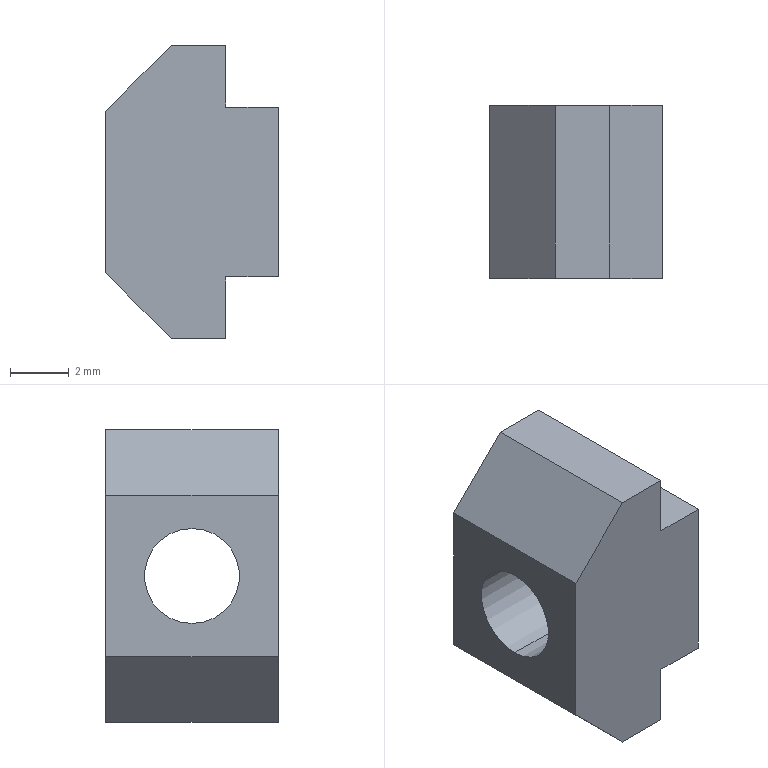Part | STEP file | PN_0018_T-slot nut M4 | 1 solid | 16 faces | box 5.9 x 5.9 x 10 mm | volume 224.64 mm3 | plane 12 | cylinder 2 | cone 2 | commonest cylinder face diameters 3.242 x2
STEP:
#1=CARTESIAN_POINT('',(0.,0.,0.));
#2=DIRECTION('',(0.,0.,1.));
#3=DIRECTION('',(1.,0.,0.));
#4=AXIS2_PLACEMENT_3D('',#1,#2,#3);
#5=CARTESIAN_POINT('',(-3770.9,379.188,502.528));
#6=VERTEX_POINT('',#5);
#7=CARTESIAN_POINT('',(-3765.219,379.188,502.528));
#8=VERTEX_POINT('',#7);
#9=CARTESIAN_POINT('',(-3765.,379.188,502.528));
#10=DIRECTION('',(1.,0.,0.));
#11=VECTOR('',#10,1.);
#12=LINE('',#9,#11);
#13=CARTESIAN_POINT('',(-3765.,379.188,504.149));
#14=DIRECTION('',(1.,0.,0.));
#15=DIRECTION('',(0.,0.,-1.));
#16=AXIS2_PLACEMENT_3D('',#13,#14,#15);
#17=CYLINDRICAL_SURFACE('',#16,1.621);
#18=CARTESIAN_POINT('',(6.283,0.));
#19=DIRECTION('',(0.,1.));
#20=VECTOR('',#19,1.);
#21=LINE('',#18,#20);
#22=(GEOMETRIC_REPRESENTATION_CONTEXT(2)PARAMETRIC_REPRESENTATION_CONTEXT()REPRESENTATION_CONTEXT('',''));
#23=DEFINITIONAL_REPRESENTATION('',(#21),#22);
#24=PCURVE('',#17,#23);
#25=CARTESIAN_POINT('',(-3765.,379.188,504.149));
#26=DIRECTION('',(1.,0.,0.));
#27=DIRECTION('',(0.,0.,-1.));
#28=AXIS2_PLACEMENT_3D('',#25,#26,#27);
#29=CYLINDRICAL_SURFACE('',#28,1.621);
#30=CARTESIAN_POINT('',(0.,0.));
#31=DIRECTION('',(0.,1.));
#32=VECTOR('',#31,1.);
#33=LINE('',#30,#32);
#34=(GEOMETRIC_REPRESENTATION_CONTEXT(2)PARAMETRIC_REPRESENTATION_CONTEXT()REPRESENTATION_CONTEXT('',''));
#35=DEFINITIONAL_REPRESENTATION('',(#33),#34);
#36=PCURVE('',#29,#35);
#37=SURFACE_CURVE('',#12,(#24,#36),.PCURVE_S1.);
#38=EDGE_CURVE('',#6,#8,#37,.T.);
#39=ORIENTED_EDGE('',*,*,#38,.T.);
#40=CARTESIAN_POINT('',(-3765.219,379.188,505.77));
#41=VERTEX_POINT('',#40);
#42=CARTESIAN_POINT('',(-3765.219,379.188,504.149));
#43=DIRECTION('',(-1.,0.,0.));
#44=DIRECTION('',(0.,0.,-1.));
#45=AXIS2_PLACEMENT_3D('',#42,#43,#44);
#46=CIRCLE('',#45,1.621);
#47=CARTESIAN_POINT('',(6.283,-0.2188));
#48=DIRECTION('',(-1.,0.));
#49=VECTOR('',#48,1.);
#50=LINE('',#47,#49);
#51=(GEOMETRIC_REPRESENTATION_CONTEXT(2)PARAMETRIC_REPRESENTATION_CONTEXT()REPRESENTATION_CONTEXT('',''));
#52=DEFINITIONAL_REPRESENTATION('',(#50),#51);
#53=PCURVE('',#17,#52);
#54=CARTESIAN_POINT('',(-3765.,379.188,504.149));
#55=DIRECTION('',(1.,0.,0.));
#56=DIRECTION('',(0.,0.,-1.));
#57=AXIS2_PLACEMENT_3D('',#54,#55,#56);
#58=CONICAL_SURFACE('',#57,2.,1.047);
#59=CARTESIAN_POINT('',(6.283,-0.2188));
#60=DIRECTION('',(-1.,0.));
#61=VECTOR('',#60,1.);
#62=LINE('',#59,#61);
#63=(GEOMETRIC_REPRESENTATION_CONTEXT(2)PARAMETRIC_REPRESENTATION_CONTEXT()REPRESENTATION_CONTEXT('',''));
#64=DEFINITIONAL_REPRESENTATION('',(#62),#63);
#65=PCURVE('',#58,#64);
#66=SURFACE_CURVE('',#46,(#53,#65),.PCURVE_S1.);
#67=EDGE_CURVE('',#8,#41,#66,.T.);
#68=ORIENTED_EDGE('',*,*,#67,.T.);
#69=CARTESIAN_POINT('',(-3770.9,379.188,505.77));
#70=VERTEX_POINT('',#69);
#71=CARTESIAN_POINT('',(-3765.,379.188,505.77));
#72=DIRECTION('',(1.,0.,0.));
#73=VECTOR('',#72,1.);
#74=LINE('',#71,#73);
#75=CARTESIAN_POINT('',(3.142,0.));
#76=DIRECTION('',(0.,1.));
#77=VECTOR('',#76,1.);
#78=LINE('',#75,#77);
#79=(GEOMETRIC_REPRESENTATION_CONTEXT(2)PARAMETRIC_REPRESENTATION_CONTEXT()REPRESENTATION_CONTEXT('',''));
#80=DEFINITIONAL_REPRESENTATION('',(#78),#79);
#81=PCURVE('',#17,#80);
#82=CARTESIAN_POINT('',(3.142,0.));
#83=DIRECTION('',(0.,1.));
#84=VECTOR('',#83,1.);
#85=LINE('',#82,#84);
#86=(GEOMETRIC_REPRESENTATION_CONTEXT(2)PARAMETRIC_REPRESENTATION_CONTEXT()REPRESENTATION_CONTEXT('',''));
#87=DEFINITIONAL_REPRESENTATION('',(#85),#86);
#88=PCURVE('',#29,#87);
#89=SURFACE_CURVE('',#74,(#81,#88),.PCURVE_S1.);
#90=EDGE_CURVE('',#70,#41,#89,.T.);
#91=ORIENTED_EDGE('',*,*,#90,.F.);
#92=CARTESIAN_POINT('',(-3770.9,379.188,504.149));
#93=DIRECTION('',(1.,0.,0.));
#94=DIRECTION('',(0.,0.,-1.));
#95=AXIS2_PLACEMENT_3D('',#92,#93,#94);
#96=CIRCLE('',#95,1.621);
#97=CARTESIAN_POINT('',(0.,-5.9));
#98=DIRECTION('',(1.,0.));
#99=VECTOR('',#98,1.);
#100=LINE('',#97,#99);
#101=(GEOMETRIC_REPRESENTATION_CONTEXT(2)PARAMETRIC_REPRESENTATION_CONTEXT()REPRESENTATION_CONTEXT('',''));
#102=DEFINITIONAL_REPRESENTATION('',(#100),#101);
#103=PCURVE('',#17,#102);
#104=CARTESIAN_POINT('',(-3770.9,376.238,501.392));
#105=DIRECTION('',(-1.,0.,0.));
#106=DIRECTION('',(0.,0.,1.));
#107=AXIS2_PLACEMENT_3D('',#104,#105,#106);
#108=PLANE('',#107);
#109=CARTESIAN_POINT('',(1.135,2.95));
#110=CARTESIAN_POINT('',(1.135,5.758));
#111=CARTESIAN_POINT('',(3.567,4.354));
#112=CARTESIAN_POINT('',(5.998,2.95));
#113=CARTESIAN_POINT('',(3.567,1.546));
#114=CARTESIAN_POINT('',(1.135,0.1423));
#115=CARTESIAN_POINT('',(1.135,2.95));
#116=(BOUNDED_CURVE()B_SPLINE_CURVE(2,(#109,#110,#111,#112,#113,#114,#115),.UNSPECIFIED.,.T.,.F.)B_SPLINE_CURVE_WITH_KNOTS((1,2,2,2,2,1),(-2.094,0.,2.094,4.189,6.283,8.378),.UNSPECIFIED.)CURVE()GEOMETRIC_REPRESENTATION_ITEM()RATIONAL_B_SPLINE_CURVE((1.,0.5,1.,0.5,1.,0.5,1.))REPRESENTATION_ITEM(''));
#117=(GEOMETRIC_REPRESENTATION_CONTEXT(2)PARAMETRIC_REPRESENTATION_CONTEXT()REPRESENTATION_CONTEXT('',''));
#118=DEFINITIONAL_REPRESENTATION('',(#116),#117);
#119=PCURVE('',#108,#118);
#120=SURFACE_CURVE('',#96,(#103,#119),.PCURVE_S1.);
#121=EDGE_CURVE('',#70,#6,#120,.T.);
#122=ORIENTED_EDGE('',*,*,#121,.T.);
#123=EDGE_LOOP('',(#39,#68,#91,#122));
#124=FACE_BOUND('',#123,.F.);
#125=ADVANCED_FACE('',(#124),#17,.F.);
#126=CARTESIAN_POINT('',(-3765.,379.188,502.149));
#127=VERTEX_POINT('',#126);
#128=CARTESIAN_POINT('',(-3765.,379.188,502.149));
#129=DIRECTION('',(0.5,0.,-0.866));
#130=VECTOR('',#129,1.);
#131=LINE('',#128,#130);
#132=CARTESIAN_POINT('',(6.283,0.));
#133=DIRECTION('',(0.,1.));
#134=VECTOR('',#133,1.);
#135=LINE('',#132,#134);
#136=(GEOMETRIC_REPRESENTATION_CONTEXT(2)PARAMETRIC_REPRESENTATION_CONTEXT()REPRESENTATION_CONTEXT('',''));
#137=DEFINITIONAL_REPRESENTATION('',(#135),#136);
#138=PCURVE('',#58,#137);
#139=CARTESIAN_POINT('',(-3765.,379.188,504.149));
#140=DIRECTION('',(1.,0.,0.));
#141=DIRECTION('',(0.,0.,-1.));
#142=AXIS2_PLACEMENT_3D('',#139,#140,#141);
#143=CONICAL_SURFACE('',#142,2.,1.047);
#144=CARTESIAN_POINT('',(0.,0.));
#145=DIRECTION('',(0.,1.));
#146=VECTOR('',#145,1.);
#147=LINE('',#144,#146);
#148=(GEOMETRIC_REPRESENTATION_CONTEXT(2)PARAMETRIC_REPRESENTATION_CONTEXT()REPRESENTATION_CONTEXT('',''));
#149=DEFINITIONAL_REPRESENTATION('',(#147),#148);
#150=PCURVE('',#143,#149);
#151=SURFACE_CURVE('',#131,(#138,#150),.PCURVE_S1.);
#152=EDGE_CURVE('',#8,#127,#151,.T.);
#153=ORIENTED_EDGE('',*,*,#152,.T.);
#154=CARTESIAN_POINT('',(-3765.,379.188,506.149));
#155=VERTEX_POINT('',#154);
#156=CARTESIAN_POINT('',(-3765.,379.188,504.149));
#157=DIRECTION('',(-1.,0.,0.));
#158=DIRECTION('',(0.,0.,-1.));
#159=AXIS2_PLACEMENT_3D('',#156,#157,#158);
#160=CIRCLE('',#159,2.);
#161=CARTESIAN_POINT('',(6.283,0.));
#162=DIRECTION('',(-1.,0.));
#163=VECTOR('',#162,1.);
#164=LINE('',#161,#163);
#165=(GEOMETRIC_REPRESENTATION_CONTEXT(2)PARAMETRIC_REPRESENTATION_CONTEXT()REPRESENTATION_CONTEXT('',''));
#166=DEFINITIONAL_REPRESENTATION('',(#164),#165);
#167=PCURVE('',#58,#166);
#168=CARTESIAN_POINT('',(-3765.,376.238,509.149));
#169=DIRECTION('',(1.,0.,0.));
#170=DIRECTION('',(0.,0.,-1.));
#171=AXIS2_PLACEMENT_3D('',#168,#169,#170);
#172=PLANE('',#171);
#173=CARTESIAN_POINT('',(7.,2.95));
#174=CARTESIAN_POINT('',(7.,-0.5141));
#175=CARTESIAN_POINT('',(4.,1.218));
#176=CARTESIAN_POINT('',(1.,2.95));
#177=CARTESIAN_POINT('',(4.,4.682));
#178=CARTESIAN_POINT('',(7.,6.414));
#179=CARTESIAN_POINT('',(7.,2.95));
#180=(BOUNDED_CURVE()B_SPLINE_CURVE(2,(#173,#174,#175,#176,#177,#178,#179),.UNSPECIFIED.,.T.,.F.)B_SPLINE_CURVE_WITH_KNOTS((1,2,2,2,2,1),(-2.094,0.,2.094,4.189,6.283,8.378),.UNSPECIFIED.)CURVE()GEOMETRIC_REPRESENTATION_ITEM()RATIONAL_B_SPLINE_CURVE((1.,0.5,1.,0.5,1.,0.5,1.))REPRESENTATION_ITEM(''));
#181=(GEOMETRIC_REPRESENTATION_CONTEXT(2)PARAMETRIC_REPRESENTATION_CONTEXT()REPRESENTATION_CONTEXT('',''));
#182=DEFINITIONAL_REPRESENTATION('',(#180),#181);
#183=PCURVE('',#172,#182);
#184=SURFACE_CURVE('',#160,(#167,#183),.PCURVE_S1.);
#185=EDGE_CURVE('',#127,#155,#184,.T.);
#186=ORIENTED_EDGE('',*,*,#185,.T.);
#187=CARTESIAN_POINT('',(-3765.,379.188,506.149));
#188=DIRECTION('',(0.5,0.,0.866));
#189=VECTOR('',#188,1.);
#190=LINE('',#187,#189);
#191=CARTESIAN_POINT('',(3.142,0.));
#192=DIRECTION('',(0.,1.));
#193=VECTOR('',#192,1.);
#194=LINE('',#191,#193);
#195=(GEOMETRIC_REPRESENTATION_CONTEXT(2)PARAMETRIC_REPRESENTATION_CONTEXT()REPRESENTATION_CONTEXT('',''));
#196=DEFINITIONAL_REPRESENTATION('',(#194),#195);
#197=PCURVE('',#58,#196);
#198=CARTESIAN_POINT('',(3.142,0.));
#199=DIRECTION('',(0.,1.));
#200=VECTOR('',#199,1.);
#201=LINE('',#198,#200);
#202=(GEOMETRIC_REPRESENTATION_CONTEXT(2)PARAMETRIC_REPRESENTATION_CONTEXT()REPRESENTATION_CONTEXT('',''));
#203=DEFINITIONAL_REPRESENTATION('',(#201),#202);
#204=PCURVE('',#143,#203);
#205=SURFACE_CURVE('',#190,(#197,#204),.PCURVE_S1.);
#206=EDGE_CURVE('',#41,#155,#205,.T.);
#207=ORIENTED_EDGE('',*,*,#206,.F.);
#208=ORIENTED_EDGE('',*,*,#67,.F.);
#209=EDGE_LOOP('',(#153,#186,#207,#208));
#210=FACE_BOUND('',#209,.F.);
#211=ADVANCED_FACE('',(#210),#58,.F.);
#212=CARTESIAN_POINT('',(-3768.656,376.238,499.149));
#213=VERTEX_POINT('',#212);
#214=CARTESIAN_POINT('',(-3766.8,376.238,499.149));
#215=VERTEX_POINT('',#214);
#216=CARTESIAN_POINT('',(0.,376.238,499.149));
#217=DIRECTION('',(1.,0.,0.));
#218=VECTOR('',#217,1.);
#219=LINE('',#216,#218);
#220=CARTESIAN_POINT('',(0.,376.238,0.));
#221=DIRECTION('',(0.,-1.,0.));
#222=DIRECTION('',(0.,0.,-1.));
#223=AXIS2_PLACEMENT_3D('',#220,#221,#222);
#224=PLANE('',#223);
#225=CARTESIAN_POINT('',(-499.149,0.));
#226=DIRECTION('',(0.,1.));
#227=VECTOR('',#226,1.);
#228=LINE('',#225,#227);
#229=(GEOMETRIC_REPRESENTATION_CONTEXT(2)PARAMETRIC_REPRESENTATION_CONTEXT()REPRESENTATION_CONTEXT('',''));
#230=DEFINITIONAL_REPRESENTATION('',(#228),#229);
#231=PCURVE('',#224,#230);
#232=CARTESIAN_POINT('',(-3765.,376.238,499.149));
#233=DIRECTION('',(0.,0.,-1.));
#234=DIRECTION('',(-1.,0.,0.));
#235=AXIS2_PLACEMENT_3D('',#232,#233,#234);
#236=PLANE('',#235);
#237=CARTESIAN_POINT('',(-3765.,0.));
#238=DIRECTION('',(-1.,0.));
#239=VECTOR('',#238,1.);
#240=LINE('',#237,#239);
#241=(GEOMETRIC_REPRESENTATION_CONTEXT(2)PARAMETRIC_REPRESENTATION_CONTEXT()REPRESENTATION_CONTEXT('',''));
#242=DEFINITIONAL_REPRESENTATION('',(#240),#241);
#243=PCURVE('',#236,#242);
#244=SURFACE_CURVE('',#219,(#231,#243),.PCURVE_S1.);
#245=EDGE_CURVE('',#213,#215,#244,.T.);
#246=ORIENTED_EDGE('',*,*,#245,.T.);
#247=CARTESIAN_POINT('',(-3766.8,376.238,501.249));
#248=VERTEX_POINT('',#247);
#249=CARTESIAN_POINT('',(-3766.8,376.238,0.));
#250=DIRECTION('',(0.,0.,1.));
#251=VECTOR('',#250,1.);
#252=LINE('',#249,#251);
#253=CARTESIAN_POINT('',(0.,-3766.8));
#254=DIRECTION('',(-1.,0.));
#255=VECTOR('',#254,1.);
#256=LINE('',#253,#255);
#257=(GEOMETRIC_REPRESENTATION_CONTEXT(2)PARAMETRIC_REPRESENTATION_CONTEXT()REPRESENTATION_CONTEXT('',''));
#258=DEFINITIONAL_REPRESENTATION('',(#256),#257);
#259=PCURVE('',#224,#258);
#260=CARTESIAN_POINT('',(-3766.8,382.138,501.249));
#261=DIRECTION('',(-1.,0.,0.));
#262=DIRECTION('',(0.,0.,1.));
#263=AXIS2_PLACEMENT_3D('',#260,#261,#262);
#264=PLANE('',#263);
#265=CARTESIAN_POINT('',(-501.249,-5.9));
#266=DIRECTION('',(1.,0.));
#267=VECTOR('',#266,1.);
#268=LINE('',#265,#267);
#269=(GEOMETRIC_REPRESENTATION_CONTEXT(2)PARAMETRIC_REPRESENTATION_CONTEXT()REPRESENTATION_CONTEXT('',''));
#270=DEFINITIONAL_REPRESENTATION('',(#268),#269);
#271=PCURVE('',#264,#270);
#272=SURFACE_CURVE('',#252,(#259,#271),.PCURVE_S1.);
#273=EDGE_CURVE('',#215,#248,#272,.T.);
#274=ORIENTED_EDGE('',*,*,#273,.T.);
#275=CARTESIAN_POINT('',(-3765.,376.238,501.249));
#276=VERTEX_POINT('',#275);
#277=CARTESIAN_POINT('',(0.,376.238,501.249));
#278=DIRECTION('',(1.,0.,0.));
#279=VECTOR('',#278,1.);
#280=LINE('',#277,#279);
#281=CARTESIAN_POINT('',(-501.249,0.));
#282=DIRECTION('',(0.,1.));
#283=VECTOR('',#282,1.);
#284=LINE('',#281,#283);
#285=(GEOMETRIC_REPRESENTATION_CONTEXT(2)PARAMETRIC_REPRESENTATION_CONTEXT()REPRESENTATION_CONTEXT('',''));
#286=DEFINITIONAL_REPRESENTATION('',(#284),#285);
#287=PCURVE('',#224,#286);
#288=CARTESIAN_POINT('',(-3765.,382.138,501.249));
#289=DIRECTION('',(0.,0.,1.));
#290=DIRECTION('',(1.,0.,0.));
#291=AXIS2_PLACEMENT_3D('',#288,#289,#290);
#292=PLANE('',#291);
#293=CARTESIAN_POINT('',(3765.,-5.9));
#294=DIRECTION('',(1.,0.));
#295=VECTOR('',#294,1.);
#296=LINE('',#293,#295);
#297=(GEOMETRIC_REPRESENTATION_CONTEXT(2)PARAMETRIC_REPRESENTATION_CONTEXT()REPRESENTATION_CONTEXT('',''));
#298=DEFINITIONAL_REPRESENTATION('',(#296),#297);
#299=PCURVE('',#292,#298);
#300=SURFACE_CURVE('',#280,(#287,#299),.PCURVE_S1.);
#301=EDGE_CURVE('',#248,#276,#300,.T.);
#302=ORIENTED_EDGE('',*,*,#301,.T.);
#303=CARTESIAN_POINT('',(-3765.,376.238,507.049));
#304=VERTEX_POINT('',#303);
#305=CARTESIAN_POINT('',(-3765.,376.238,0.));
#306=DIRECTION('',(0.,0.,1.));
#307=VECTOR('',#306,1.);
#308=LINE('',#305,#307);
#309=CARTESIAN_POINT('',(0.,-3765.));
#310=DIRECTION('',(-1.,0.));
#311=VECTOR('',#310,1.);
#312=LINE('',#309,#311);
#313=(GEOMETRIC_REPRESENTATION_CONTEXT(2)PARAMETRIC_REPRESENTATION_CONTEXT()REPRESENTATION_CONTEXT('',''));
#314=DEFINITIONAL_REPRESENTATION('',(#312),#313);
#315=PCURVE('',#224,#314);
#316=CARTESIAN_POINT('',(509.149,0.));
#317=DIRECTION('',(-1.,0.));
#318=VECTOR('',#317,1.);
#319=LINE('',#316,#318);
#320=(GEOMETRIC_REPRESENTATION_CONTEXT(2)PARAMETRIC_REPRESENTATION_CONTEXT()REPRESENTATION_CONTEXT('',''));
#321=DEFINITIONAL_REPRESENTATION('',(#319),#320);
#322=PCURVE('',#172,#321);
#323=SURFACE_CURVE('',#308,(#315,#322),.PCURVE_S1.);
#324=EDGE_CURVE('',#276,#304,#323,.T.);
#325=ORIENTED_EDGE('',*,*,#324,.T.);
#326=CARTESIAN_POINT('',(-3766.8,376.238,507.049));
#327=VERTEX_POINT('',#326);
#328=CARTESIAN_POINT('',(0.,376.238,507.049));
#329=DIRECTION('',(-1.,0.,0.));
#330=VECTOR('',#329,1.);
#331=LINE('',#328,#330);
#332=CARTESIAN_POINT('',(-507.049,0.));
#333=DIRECTION('',(0.,-1.));
#334=VECTOR('',#333,1.);
#335=LINE('',#332,#334);
#336=(GEOMETRIC_REPRESENTATION_CONTEXT(2)PARAMETRIC_REPRESENTATION_CONTEXT()REPRESENTATION_CONTEXT('',''));
#337=DEFINITIONAL_REPRESENTATION('',(#335),#336);
#338=PCURVE('',#224,#337);
#339=CARTESIAN_POINT('',(-3766.8,382.138,507.049));
#340=DIRECTION('',(0.,0.,-1.));
#341=DIRECTION('',(-1.,0.,0.));
#342=AXIS2_PLACEMENT_3D('',#339,#340,#341);
#343=PLANE('',#342);
#344=CARTESIAN_POINT('',(-3766.8,-5.9));
#345=DIRECTION('',(1.,0.));
#346=VECTOR('',#345,1.);
#347=LINE('',#344,#346);
#348=(GEOMETRIC_REPRESENTATION_CONTEXT(2)PARAMETRIC_REPRESENTATION_CONTEXT()REPRESENTATION_CONTEXT('',''));
#349=DEFINITIONAL_REPRESENTATION('',(#347),#348);
#350=PCURVE('',#343,#349);
#351=SURFACE_CURVE('',#331,(#338,#350),.PCURVE_S1.);
#352=EDGE_CURVE('',#304,#327,#351,.T.);
#353=ORIENTED_EDGE('',*,*,#352,.T.);
#354=CARTESIAN_POINT('',(-3766.8,376.238,509.149));
#355=VERTEX_POINT('',#354);
#356=CARTESIAN_POINT('',(-3766.8,376.238,0.));
#357=DIRECTION('',(0.,0.,1.));
#358=VECTOR('',#357,1.);
#359=LINE('',#356,#358);
#360=CARTESIAN_POINT('',(0.,-3766.8));
#361=DIRECTION('',(-1.,0.));
#362=VECTOR('',#361,1.);
#363=LINE('',#360,#362);
#364=(GEOMETRIC_REPRESENTATION_CONTEXT(2)PARAMETRIC_REPRESENTATION_CONTEXT()REPRESENTATION_CONTEXT('',''));
#365=DEFINITIONAL_REPRESENTATION('',(#363),#364);
#366=PCURVE('',#224,#365);
#367=CARTESIAN_POINT('',(-3766.8,382.138,509.149));
#368=DIRECTION('',(-1.,0.,0.));
#369=DIRECTION('',(0.,0.,1.));
#370=AXIS2_PLACEMENT_3D('',#367,#368,#369);
#371=PLANE('',#370);
#372=CARTESIAN_POINT('',(-509.149,-5.9));
#373=DIRECTION('',(1.,0.));
#374=VECTOR('',#373,1.);
#375=LINE('',#372,#374);
#376=(GEOMETRIC_REPRESENTATION_CONTEXT(2)PARAMETRIC_REPRESENTATION_CONTEXT()REPRESENTATION_CONTEXT('',''));
#377=DEFINITIONAL_REPRESENTATION('',(#375),#376);
#378=PCURVE('',#371,#377);
#379=SURFACE_CURVE('',#359,(#366,#378),.PCURVE_S1.);
#380=EDGE_CURVE('',#327,#355,#379,.T.);
#381=ORIENTED_EDGE('',*,*,#380,.T.);
#382=CARTESIAN_POINT('',(-3768.656,376.238,509.149));
#383=VERTEX_POINT('',#382);
#384=CARTESIAN_POINT('',(0.,376.238,509.149));
#385=DIRECTION('',(-1.,0.,0.));
#386=VECTOR('',#385,1.);
#387=LINE('',#384,#386);
#388=CARTESIAN_POINT('',(-509.149,0.));
#389=DIRECTION('',(0.,-1.));
#390=VECTOR('',#389,1.);
#391=LINE('',#388,#390);
#392=(GEOMETRIC_REPRESENTATION_CONTEXT(2)PARAMETRIC_REPRESENTATION_CONTEXT()REPRESENTATION_CONTEXT('',''));
#393=DEFINITIONAL_REPRESENTATION('',(#391),#392);
#394=PCURVE('',#224,#393);
#395=CARTESIAN_POINT('',(-3768.656,376.238,509.149));
#396=DIRECTION('',(0.,0.,1.));
#397=DIRECTION('',(1.,0.,0.));
#398=AXIS2_PLACEMENT_3D('',#395,#396,#397);
#399=PLANE('',#398);
#400=CARTESIAN_POINT('',(3768.656,0.));
#401=DIRECTION('',(-1.,0.));
#402=VECTOR('',#401,1.);
#403=LINE('',#400,#402);
#404=(GEOMETRIC_REPRESENTATION_CONTEXT(2)PARAMETRIC_REPRESENTATION_CONTEXT()REPRESENTATION_CONTEXT('',''));
#405=DEFINITIONAL_REPRESENTATION('',(#403),#404);
#406=PCURVE('',#399,#405);
#407=SURFACE_CURVE('',#387,(#394,#406),.PCURVE_S1.);
#408=EDGE_CURVE('',#355,#383,#407,.T.);
#409=ORIENTED_EDGE('',*,*,#408,.T.);
#410=CARTESIAN_POINT('',(-3770.9,376.238,506.905));
#411=VERTEX_POINT('',#410);
#412=CARTESIAN_POINT('',(-3768.656,376.238,509.149));
#413=DIRECTION('',(-0.7071,0.,-0.7071));
#414=VECTOR('',#413,1.);
#415=LINE('',#412,#414);
#416=CARTESIAN_POINT('',(-509.149,-3768.656));
#417=DIRECTION('',(0.7071,-0.7071));
#418=VECTOR('',#417,1.);
#419=LINE('',#416,#418);
#420=(GEOMETRIC_REPRESENTATION_CONTEXT(2)PARAMETRIC_REPRESENTATION_CONTEXT()REPRESENTATION_CONTEXT('',''));
#421=DEFINITIONAL_REPRESENTATION('',(#419),#420);
#422=PCURVE('',#224,#421);
#423=CARTESIAN_POINT('',(-3770.9,376.238,506.905));
#424=DIRECTION('',(-0.7071,0.,0.7071));
#425=DIRECTION('',(0.7071,0.,0.7071));
#426=AXIS2_PLACEMENT_3D('',#423,#424,#425);
#427=PLANE('',#426);
#428=CARTESIAN_POINT('',(3.173,0.));
#429=DIRECTION('',(-1.,0.));
#430=VECTOR('',#429,1.);
#431=LINE('',#428,#430);
#432=(GEOMETRIC_REPRESENTATION_CONTEXT(2)PARAMETRIC_REPRESENTATION_CONTEXT()REPRESENTATION_CONTEXT('',''));
#433=DEFINITIONAL_REPRESENTATION('',(#431),#432);
#434=PCURVE('',#427,#433);
#435=SURFACE_CURVE('',#415,(#422,#434),.PCURVE_S1.);
#436=EDGE_CURVE('',#383,#411,#435,.T.);
#437=ORIENTED_EDGE('',*,*,#436,.T.);
#438=CARTESIAN_POINT('',(-3770.9,376.238,501.392));
#439=VERTEX_POINT('',#438);
#440=CARTESIAN_POINT('',(-3770.9,376.238,0.));
#441=DIRECTION('',(0.,0.,-1.));
#442=VECTOR('',#441,1.);
#443=LINE('',#440,#442);
#444=CARTESIAN_POINT('',(0.,-3770.9));
#445=DIRECTION('',(1.,0.));
#446=VECTOR('',#445,1.);
#447=LINE('',#444,#446);
#448=(GEOMETRIC_REPRESENTATION_CONTEXT(2)PARAMETRIC_REPRESENTATION_CONTEXT()REPRESENTATION_CONTEXT('',''));
#449=DEFINITIONAL_REPRESENTATION('',(#447),#448);
#450=PCURVE('',#224,#449);
#451=CARTESIAN_POINT('',(-501.392,0.));
#452=DIRECTION('',(-1.,0.));
#453=VECTOR('',#452,1.);
#454=LINE('',#451,#453);
#455=(GEOMETRIC_REPRESENTATION_CONTEXT(2)PARAMETRIC_REPRESENTATION_CONTEXT()REPRESENTATION_CONTEXT('',''));
#456=DEFINITIONAL_REPRESENTATION('',(#454),#455);
#457=PCURVE('',#108,#456);
#458=SURFACE_CURVE('',#443,(#450,#457),.PCURVE_S1.);
#459=EDGE_CURVE('',#411,#439,#458,.T.);
#460=ORIENTED_EDGE('',*,*,#459,.T.);
#461=CARTESIAN_POINT('',(-3770.9,376.238,501.392));
#462=DIRECTION('',(0.7071,0.,-0.7071));
#463=VECTOR('',#462,1.);
#464=LINE('',#461,#463);
#465=CARTESIAN_POINT('',(-501.392,-3770.9));
#466=DIRECTION('',(0.7071,0.7071));
#467=VECTOR('',#466,1.);
#468=LINE('',#465,#467);
#469=(GEOMETRIC_REPRESENTATION_CONTEXT(2)PARAMETRIC_REPRESENTATION_CONTEXT()REPRESENTATION_CONTEXT('',''));
#470=DEFINITIONAL_REPRESENTATION('',(#468),#469);
#471=PCURVE('',#224,#470);
#472=CARTESIAN_POINT('',(-3768.656,376.238,499.149));
#473=DIRECTION('',(-0.7071,0.,-0.7071));
#474=DIRECTION('',(-0.7071,0.,0.7071));
#475=AXIS2_PLACEMENT_3D('',#472,#473,#474);
#476=PLANE('',#475);
#477=CARTESIAN_POINT('',(3.173,0.));
#478=DIRECTION('',(-1.,0.));
#479=VECTOR('',#478,1.);
#480=LINE('',#477,#479);
#481=(GEOMETRIC_REPRESENTATION_CONTEXT(2)PARAMETRIC_REPRESENTATION_CONTEXT()REPRESENTATION_CONTEXT('',''));
#482=DEFINITIONAL_REPRESENTATION('',(#480),#481);
#483=PCURVE('',#476,#482);
#484=SURFACE_CURVE('',#464,(#471,#483),.PCURVE_S1.);
#485=EDGE_CURVE('',#439,#213,#484,.T.);
#486=ORIENTED_EDGE('',*,*,#485,.T.);
#487=EDGE_LOOP('',(#246,#274,#302,#325,#353,#381,#409,#437,#460,#486));
#488=FACE_BOUND('',#487,.T.);
#489=ADVANCED_FACE('',(#488),#224,.T.);
#490=CARTESIAN_POINT('',(-3766.8,382.138,499.149));
#491=VERTEX_POINT('',#490);
#492=CARTESIAN_POINT('',(-3766.8,382.138,499.149));
#493=DIRECTION('',(0.,-1.,0.));
#494=VECTOR('',#493,1.);
#495=LINE('',#492,#494);
#496=CARTESIAN_POINT('',(-2.1,0.));
#497=DIRECTION('',(0.,-1.));
#498=VECTOR('',#497,1.);
#499=LINE('',#496,#498);
#500=(GEOMETRIC_REPRESENTATION_CONTEXT(2)PARAMETRIC_REPRESENTATION_CONTEXT()REPRESENTATION_CONTEXT('',''));
#501=DEFINITIONAL_REPRESENTATION('',(#499),#500);
#502=PCURVE('',#264,#501);
#503=CARTESIAN_POINT('',(1.8,5.9));
#504=DIRECTION('',(0.,-1.));
#505=VECTOR('',#504,1.);
#506=LINE('',#503,#505);
#507=(GEOMETRIC_REPRESENTATION_CONTEXT(2)PARAMETRIC_REPRESENTATION_CONTEXT()REPRESENTATION_CONTEXT('',''));
#508=DEFINITIONAL_REPRESENTATION('',(#506),#507);
#509=PCURVE('',#236,#508);
#510=SURFACE_CURVE('',#495,(#502,#509),.PCURVE_S1.);
#511=EDGE_CURVE('',#491,#215,#510,.T.);
#512=ORIENTED_EDGE('',*,*,#511,.F.);
#513=CARTESIAN_POINT('',(-3766.8,382.138,501.249));
#514=VERTEX_POINT('',#513);
#515=CARTESIAN_POINT('',(-3766.8,382.138,501.249));
#516=DIRECTION('',(0.,0.,-1.));
#517=VECTOR('',#516,1.);
#518=LINE('',#515,#517);
#519=CARTESIAN_POINT('',(0.,0.));
#520=DIRECTION('',(-1.,0.));
#521=VECTOR('',#520,1.);
#522=LINE('',#519,#521);
#523=(GEOMETRIC_REPRESENTATION_CONTEXT(2)PARAMETRIC_REPRESENTATION_CONTEXT()REPRESENTATION_CONTEXT('',''));
#524=DEFINITIONAL_REPRESENTATION('',(#522),#523);
#525=PCURVE('',#264,#524);
#526=CARTESIAN_POINT('',(0.,382.138,0.));
#527=DIRECTION('',(0.,-1.,0.));
#528=DIRECTION('',(0.,0.,-1.));
#529=AXIS2_PLACEMENT_3D('',#526,#527,#528);
#530=PLANE('',#529);
#531=CARTESIAN_POINT('',(-501.249,-3766.8));
#532=DIRECTION('',(1.,0.));
#533=VECTOR('',#532,1.);
#534=LINE('',#531,#533);
#535=(GEOMETRIC_REPRESENTATION_CONTEXT(2)PARAMETRIC_REPRESENTATION_CONTEXT()REPRESENTATION_CONTEXT('',''));
#536=DEFINITIONAL_REPRESENTATION('',(#534),#535);
#537=PCURVE('',#530,#536);
#538=SURFACE_CURVE('',#518,(#525,#537),.PCURVE_S1.);
#539=EDGE_CURVE('',#514,#491,#538,.T.);
#540=ORIENTED_EDGE('',*,*,#539,.F.);
#541=CARTESIAN_POINT('',(-3766.8,382.138,501.249));
#542=DIRECTION('',(0.,1.,0.));
#543=VECTOR('',#542,1.);
#544=LINE('',#541,#543);
#545=CARTESIAN_POINT('',(0.,0.));
#546=DIRECTION('',(0.,1.));
#547=VECTOR('',#546,1.);
#548=LINE('',#545,#547);
#549=(GEOMETRIC_REPRESENTATION_CONTEXT(2)PARAMETRIC_REPRESENTATION_CONTEXT()REPRESENTATION_CONTEXT('',''));
#550=DEFINITIONAL_REPRESENTATION('',(#548),#549);
#551=PCURVE('',#264,#550);
#552=CARTESIAN_POINT('',(-1.8,0.));
#553=DIRECTION('',(0.,1.));
#554=VECTOR('',#553,1.);
#555=LINE('',#552,#554);
#556=(GEOMETRIC_REPRESENTATION_CONTEXT(2)PARAMETRIC_REPRESENTATION_CONTEXT()REPRESENTATION_CONTEXT('',''));
#557=DEFINITIONAL_REPRESENTATION('',(#555),#556);
#558=PCURVE('',#292,#557);
#559=SURFACE_CURVE('',#544,(#551,#558),.PCURVE_S1.);
#560=EDGE_CURVE('',#248,#514,#559,.T.);
#561=ORIENTED_EDGE('',*,*,#560,.F.);
#562=ORIENTED_EDGE('',*,*,#273,.F.);
#563=EDGE_LOOP('',(#512,#540,#561,#562));
#564=FACE_BOUND('',#563,.T.);
#565=ADVANCED_FACE('',(#564),#264,.F.);
#566=CARTESIAN_POINT('',(-3768.656,382.138,499.149));
#567=VERTEX_POINT('',#566);
#568=CARTESIAN_POINT('',(-3768.656,376.238,499.149));
#569=DIRECTION('',(0.,1.,0.));
#570=VECTOR('',#569,1.);
#571=LINE('',#568,#570);
#572=CARTESIAN_POINT('',(3.656,0.));
#573=DIRECTION('',(0.,1.));
#574=VECTOR('',#573,1.);
#575=LINE('',#572,#574);
#576=(GEOMETRIC_REPRESENTATION_CONTEXT(2)PARAMETRIC_REPRESENTATION_CONTEXT()REPRESENTATION_CONTEXT('',''));
#577=DEFINITIONAL_REPRESENTATION('',(#575),#576);
#578=PCURVE('',#236,#577);
#579=CARTESIAN_POINT('',(0.,0.));
#580=DIRECTION('',(0.,1.));
#581=VECTOR('',#580,1.);
#582=LINE('',#579,#581);
#583=(GEOMETRIC_REPRESENTATION_CONTEXT(2)PARAMETRIC_REPRESENTATION_CONTEXT()REPRESENTATION_CONTEXT('',''));
#584=DEFINITIONAL_REPRESENTATION('',(#582),#583);
#585=PCURVE('',#476,#584);
#586=SURFACE_CURVE('',#571,(#578,#585),.PCURVE_S1.);
#587=EDGE_CURVE('',#213,#567,#586,.T.);
#588=ORIENTED_EDGE('',*,*,#587,.T.);
#589=CARTESIAN_POINT('',(-3765.,382.138,499.149));
#590=DIRECTION('',(1.,0.,0.));
#591=VECTOR('',#590,1.);
#592=LINE('',#589,#591);
#593=CARTESIAN_POINT('',(0.,5.9));
#594=DIRECTION('',(-1.,0.));
#595=VECTOR('',#594,1.);
#596=LINE('',#593,#595);
#597=(GEOMETRIC_REPRESENTATION_CONTEXT(2)PARAMETRIC_REPRESENTATION_CONTEXT()REPRESENTATION_CONTEXT('',''));
#598=DEFINITIONAL_REPRESENTATION('',(#596),#597);
#599=PCURVE('',#236,#598);
#600=CARTESIAN_POINT('',(-499.149,-3765.));
#601=DIRECTION('',(0.,1.));
#602=VECTOR('',#601,1.);
#603=LINE('',#600,#602);
#604=(GEOMETRIC_REPRESENTATION_CONTEXT(2)PARAMETRIC_REPRESENTATION_CONTEXT()REPRESENTATION_CONTEXT('',''));
#605=DEFINITIONAL_REPRESENTATION('',(#603),#604);
#606=PCURVE('',#530,#605);
#607=SURFACE_CURVE('',#592,(#599,#606),.PCURVE_S1.);
#608=EDGE_CURVE('',#567,#491,#607,.T.);
#609=ORIENTED_EDGE('',*,*,#608,.T.);
#610=ORIENTED_EDGE('',*,*,#511,.T.);
#611=ORIENTED_EDGE('',*,*,#245,.F.);
#612=EDGE_LOOP('',(#588,#609,#610,#611));
#613=FACE_BOUND('',#612,.T.);
#614=ADVANCED_FACE('',(#613),#236,.T.);
#615=ORIENTED_EDGE('',*,*,#485,.F.);
#616=CARTESIAN_POINT('',(-3770.9,382.138,501.392));
#617=VERTEX_POINT('',#616);
#618=CARTESIAN_POINT('',(-3770.9,376.238,501.392));
#619=DIRECTION('',(0.,1.,0.));
#620=VECTOR('',#619,1.);
#621=LINE('',#618,#620);
#622=CARTESIAN_POINT('',(3.173,0.));
#623=DIRECTION('',(0.,1.));
#624=VECTOR('',#623,1.);
#625=LINE('',#622,#624);
#626=(GEOMETRIC_REPRESENTATION_CONTEXT(2)PARAMETRIC_REPRESENTATION_CONTEXT()REPRESENTATION_CONTEXT('',''));
#627=DEFINITIONAL_REPRESENTATION('',(#625),#626);
#628=PCURVE('',#476,#627);
#629=CARTESIAN_POINT('',(0.,0.));
#630=DIRECTION('',(0.,1.));
#631=VECTOR('',#630,1.);
#632=LINE('',#629,#631);
#633=(GEOMETRIC_REPRESENTATION_CONTEXT(2)PARAMETRIC_REPRESENTATION_CONTEXT()REPRESENTATION_CONTEXT('',''));
#634=DEFINITIONAL_REPRESENTATION('',(#632),#633);
#635=PCURVE('',#108,#634);
#636=SURFACE_CURVE('',#621,(#628,#635),.PCURVE_S1.);
#637=EDGE_CURVE('',#439,#617,#636,.T.);
#638=ORIENTED_EDGE('',*,*,#637,.T.);
#639=CARTESIAN_POINT('',(-3768.656,382.138,499.149));
#640=DIRECTION('',(0.7071,0.,-0.7071));
#641=VECTOR('',#640,1.);
#642=LINE('',#639,#641);
#643=CARTESIAN_POINT('',(0.,5.9));
#644=DIRECTION('',(-1.,0.));
#645=VECTOR('',#644,1.);
#646=LINE('',#643,#645);
#647=(GEOMETRIC_REPRESENTATION_CONTEXT(2)PARAMETRIC_REPRESENTATION_CONTEXT()REPRESENTATION_CONTEXT('',''));
#648=DEFINITIONAL_REPRESENTATION('',(#646),#647);
#649=PCURVE('',#476,#648);
#650=CARTESIAN_POINT('',(-499.149,-3768.656));
#651=DIRECTION('',(0.7071,0.7071));
#652=VECTOR('',#651,1.);
#653=LINE('',#650,#652);
#654=(GEOMETRIC_REPRESENTATION_CONTEXT(2)PARAMETRIC_REPRESENTATION_CONTEXT()REPRESENTATION_CONTEXT('',''));
#655=DEFINITIONAL_REPRESENTATION('',(#653),#654);
#656=PCURVE('',#530,#655);
#657=SURFACE_CURVE('',#642,(#649,#656),.PCURVE_S1.);
#658=EDGE_CURVE('',#617,#567,#657,.T.);
#659=ORIENTED_EDGE('',*,*,#658,.T.);
#660=ORIENTED_EDGE('',*,*,#587,.F.);
#661=EDGE_LOOP('',(#615,#638,#659,#660));
#662=FACE_BOUND('',#661,.T.);
#663=ADVANCED_FACE('',(#662),#476,.T.);
#664=ORIENTED_EDGE('',*,*,#459,.F.);
#665=CARTESIAN_POINT('',(-3770.9,382.138,506.905));
#666=VERTEX_POINT('',#665);
#667=CARTESIAN_POINT('',(-3770.9,376.238,506.905));
#668=DIRECTION('',(0.,1.,0.));
#669=VECTOR('',#668,1.);
#670=LINE('',#667,#669);
#671=CARTESIAN_POINT('',(5.513,0.));
#672=DIRECTION('',(0.,1.));
#673=VECTOR('',#672,1.);
#674=LINE('',#671,#673);
#675=(GEOMETRIC_REPRESENTATION_CONTEXT(2)PARAMETRIC_REPRESENTATION_CONTEXT()REPRESENTATION_CONTEXT('',''));
#676=DEFINITIONAL_REPRESENTATION('',(#674),#675);
#677=PCURVE('',#108,#676);
#678=CARTESIAN_POINT('',(0.,0.));
#679=DIRECTION('',(0.,1.));
#680=VECTOR('',#679,1.);
#681=LINE('',#678,#680);
#682=(GEOMETRIC_REPRESENTATION_CONTEXT(2)PARAMETRIC_REPRESENTATION_CONTEXT()REPRESENTATION_CONTEXT('',''));
#683=DEFINITIONAL_REPRESENTATION('',(#681),#682);
#684=PCURVE('',#427,#683);
#685=SURFACE_CURVE('',#670,(#677,#684),.PCURVE_S1.);
#686=EDGE_CURVE('',#411,#666,#685,.T.);
#687=ORIENTED_EDGE('',*,*,#686,.T.);
#688=CARTESIAN_POINT('',(-3770.9,382.138,501.392));
#689=DIRECTION('',(0.,0.,-1.));
#690=VECTOR('',#689,1.);
#691=LINE('',#688,#690);
#692=CARTESIAN_POINT('',(0.,5.9));
#693=DIRECTION('',(-1.,0.));
#694=VECTOR('',#693,1.);
#695=LINE('',#692,#694);
#696=(GEOMETRIC_REPRESENTATION_CONTEXT(2)PARAMETRIC_REPRESENTATION_CONTEXT()REPRESENTATION_CONTEXT('',''));
#697=DEFINITIONAL_REPRESENTATION('',(#695),#696);
#698=PCURVE('',#108,#697);
#699=CARTESIAN_POINT('',(-501.392,-3770.9));
#700=DIRECTION('',(1.,0.));
#701=VECTOR('',#700,1.);
#702=LINE('',#699,#701);
#703=(GEOMETRIC_REPRESENTATION_CONTEXT(2)PARAMETRIC_REPRESENTATION_CONTEXT()REPRESENTATION_CONTEXT('',''));
#704=DEFINITIONAL_REPRESENTATION('',(#702),#703);
#705=PCURVE('',#530,#704);
#706=SURFACE_CURVE('',#691,(#698,#705),.PCURVE_S1.);
#707=EDGE_CURVE('',#666,#617,#706,.T.);
#708=ORIENTED_EDGE('',*,*,#707,.T.);
#709=ORIENTED_EDGE('',*,*,#637,.F.);
#710=EDGE_LOOP('',(#664,#687,#708,#709));
#711=FACE_BOUND('',#710,.T.);
#712=CARTESIAN_POINT('',(-3770.9,379.188,504.149));
#713=DIRECTION('',(1.,0.,0.));
#714=DIRECTION('',(0.,0.,-1.));
#715=AXIS2_PLACEMENT_3D('',#712,#713,#714);
#716=CIRCLE('',#715,1.621);
#717=CARTESIAN_POINT('',(1.135,2.95));
#718=CARTESIAN_POINT('',(1.135,5.758));
#719=CARTESIAN_POINT('',(3.567,4.354));
#720=CARTESIAN_POINT('',(5.998,2.95));
#721=CARTESIAN_POINT('',(3.567,1.546));
#722=CARTESIAN_POINT('',(1.135,0.1423));
#723=CARTESIAN_POINT('',(1.135,2.95));
#724=(BOUNDED_CURVE()B_SPLINE_CURVE(2,(#717,#718,#719,#720,#721,#722,#723),.UNSPECIFIED.,.T.,.F.)B_SPLINE_CURVE_WITH_KNOTS((1,2,2,2,2,1),(-2.094,0.,2.094,4.189,6.283,8.378),.UNSPECIFIED.)CURVE()GEOMETRIC_REPRESENTATION_ITEM()RATIONAL_B_SPLINE_CURVE((1.,0.5,1.,0.5,1.,0.5,1.))REPRESENTATION_ITEM(''));
#725=(GEOMETRIC_REPRESENTATION_CONTEXT(2)PARAMETRIC_REPRESENTATION_CONTEXT()REPRESENTATION_CONTEXT('',''));
#726=DEFINITIONAL_REPRESENTATION('',(#724),#725);
#727=PCURVE('',#108,#726);
#728=CARTESIAN_POINT('',(0.,-5.9));
#729=DIRECTION('',(1.,0.));
#730=VECTOR('',#729,1.);
#731=LINE('',#728,#730);
#732=(GEOMETRIC_REPRESENTATION_CONTEXT(2)PARAMETRIC_REPRESENTATION_CONTEXT()REPRESENTATION_CONTEXT('',''));
#733=DEFINITIONAL_REPRESENTATION('',(#731),#732);
#734=PCURVE('',#29,#733);
#735=SURFACE_CURVE('',#716,(#727,#734),.PCURVE_S1.);
#736=EDGE_CURVE('',#6,#70,#735,.T.);
#737=ORIENTED_EDGE('',*,*,#736,.T.);
#738=ORIENTED_EDGE('',*,*,#121,.T.);
#739=EDGE_LOOP('',(#737,#738));
#740=FACE_BOUND('',#739,.T.);
#741=ADVANCED_FACE('',(#711,#740),#108,.T.);
#742=ORIENTED_EDGE('',*,*,#436,.F.);
#743=CARTESIAN_POINT('',(-3768.656,382.138,509.149));
#744=VERTEX_POINT('',#743);
#745=CARTESIAN_POINT('',(-3768.656,376.238,509.149));
#746=DIRECTION('',(0.,1.,0.));
#747=VECTOR('',#746,1.);
#748=LINE('',#745,#747);
#749=CARTESIAN_POINT('',(3.173,0.));
#750=DIRECTION('',(0.,1.));
#751=VECTOR('',#750,1.);
#752=LINE('',#749,#751);
#753=(GEOMETRIC_REPRESENTATION_CONTEXT(2)PARAMETRIC_REPRESENTATION_CONTEXT()REPRESENTATION_CONTEXT('',''));
#754=DEFINITIONAL_REPRESENTATION('',(#752),#753);
#755=PCURVE('',#427,#754);
#756=CARTESIAN_POINT('',(0.,0.));
#757=DIRECTION('',(0.,1.));
#758=VECTOR('',#757,1.);
#759=LINE('',#756,#758);
#760=(GEOMETRIC_REPRESENTATION_CONTEXT(2)PARAMETRIC_REPRESENTATION_CONTEXT()REPRESENTATION_CONTEXT('',''));
#761=DEFINITIONAL_REPRESENTATION('',(#759),#760);
#762=PCURVE('',#399,#761);
#763=SURFACE_CURVE('',#748,(#755,#762),.PCURVE_S1.);
#764=EDGE_CURVE('',#383,#744,#763,.T.);
#765=ORIENTED_EDGE('',*,*,#764,.T.);
#766=CARTESIAN_POINT('',(-3770.9,382.138,506.905));
#767=DIRECTION('',(-0.7071,0.,-0.7071));
#768=VECTOR('',#767,1.);
#769=LINE('',#766,#768);
#770=CARTESIAN_POINT('',(0.,5.9));
#771=DIRECTION('',(-1.,0.));
#772=VECTOR('',#771,1.);
#773=LINE('',#770,#772);
#774=(GEOMETRIC_REPRESENTATION_CONTEXT(2)PARAMETRIC_REPRESENTATION_CONTEXT()REPRESENTATION_CONTEXT('',''));
#775=DEFINITIONAL_REPRESENTATION('',(#773),#774);
#776=PCURVE('',#427,#775);
#777=CARTESIAN_POINT('',(-506.905,-3770.9));
#778=DIRECTION('',(0.7071,-0.7071));
#779=VECTOR('',#778,1.);
#780=LINE('',#777,#779);
#781=(GEOMETRIC_REPRESENTATION_CONTEXT(2)PARAMETRIC_REPRESENTATION_CONTEXT()REPRESENTATION_CONTEXT('',''));
#782=DEFINITIONAL_REPRESENTATION('',(#780),#781);
#783=PCURVE('',#530,#782);
#784=SURFACE_CURVE('',#769,(#776,#783),.PCURVE_S1.);
#785=EDGE_CURVE('',#744,#666,#784,.T.);
#786=ORIENTED_EDGE('',*,*,#785,.T.);
#787=ORIENTED_EDGE('',*,*,#686,.F.);
#788=EDGE_LOOP('',(#742,#765,#786,#787));
#789=FACE_BOUND('',#788,.T.);
#790=ADVANCED_FACE('',(#789),#427,.T.);
#791=ORIENTED_EDGE('',*,*,#764,.F.);
#792=ORIENTED_EDGE('',*,*,#408,.F.);
#793=CARTESIAN_POINT('',(-3766.8,382.138,509.149));
#794=VERTEX_POINT('',#793);
#795=CARTESIAN_POINT('',(-3766.8,376.238,509.149));
#796=DIRECTION('',(0.,1.,0.));
#797=VECTOR('',#796,1.);
#798=LINE('',#795,#797);
#799=CARTESIAN_POINT('',(1.856,0.));
#800=DIRECTION('',(0.,1.));
#801=VECTOR('',#800,1.);
#802=LINE('',#799,#801);
#803=(GEOMETRIC_REPRESENTATION_CONTEXT(2)PARAMETRIC_REPRESENTATION_CONTEXT()REPRESENTATION_CONTEXT('',''));
#804=DEFINITIONAL_REPRESENTATION('',(#802),#803);
#805=PCURVE('',#399,#804);
#806=CARTESIAN_POINT('',(0.,-5.9));
#807=DIRECTION('',(0.,1.));
#808=VECTOR('',#807,1.);
#809=LINE('',#806,#808);
#810=(GEOMETRIC_REPRESENTATION_CONTEXT(2)PARAMETRIC_REPRESENTATION_CONTEXT()REPRESENTATION_CONTEXT('',''));
#811=DEFINITIONAL_REPRESENTATION('',(#809),#810);
#812=PCURVE('',#371,#811);
#813=SURFACE_CURVE('',#798,(#805,#812),.PCURVE_S1.);
#814=EDGE_CURVE('',#355,#794,#813,.T.);
#815=ORIENTED_EDGE('',*,*,#814,.T.);
#816=CARTESIAN_POINT('',(-3768.656,382.138,509.149));
#817=DIRECTION('',(-1.,0.,0.));
#818=VECTOR('',#817,1.);
#819=LINE('',#816,#818);
#820=CARTESIAN_POINT('',(0.,5.9));
#821=DIRECTION('',(-1.,0.));
#822=VECTOR('',#821,1.);
#823=LINE('',#820,#822);
#824=(GEOMETRIC_REPRESENTATION_CONTEXT(2)PARAMETRIC_REPRESENTATION_CONTEXT()REPRESENTATION_CONTEXT('',''));
#825=DEFINITIONAL_REPRESENTATION('',(#823),#824);
#826=PCURVE('',#399,#825);
#827=CARTESIAN_POINT('',(-509.149,-3768.656));
#828=DIRECTION('',(0.,-1.));
#829=VECTOR('',#828,1.);
#830=LINE('',#827,#829);
#831=(GEOMETRIC_REPRESENTATION_CONTEXT(2)PARAMETRIC_REPRESENTATION_CONTEXT()REPRESENTATION_CONTEXT('',''));
#832=DEFINITIONAL_REPRESENTATION('',(#830),#831);
#833=PCURVE('',#530,#832);
#834=SURFACE_CURVE('',#819,(#826,#833),.PCURVE_S1.);
#835=EDGE_CURVE('',#794,#744,#834,.T.);
#836=ORIENTED_EDGE('',*,*,#835,.T.);
#837=EDGE_LOOP('',(#791,#792,#815,#836));
#838=FACE_BOUND('',#837,.T.);
#839=ADVANCED_FACE('',(#838),#399,.T.);
#840=CARTESIAN_POINT('',(-3766.8,382.138,507.049));
#841=VERTEX_POINT('',#840);
#842=CARTESIAN_POINT('',(-3766.8,382.138,507.049));
#843=DIRECTION('',(0.,-1.,0.));
#844=VECTOR('',#843,1.);
#845=LINE('',#842,#844);
#846=CARTESIAN_POINT('',(-2.1,0.));
#847=DIRECTION('',(0.,-1.));
#848=VECTOR('',#847,1.);
#849=LINE('',#846,#848);
#850=(GEOMETRIC_REPRESENTATION_CONTEXT(2)PARAMETRIC_REPRESENTATION_CONTEXT()REPRESENTATION_CONTEXT('',''));
#851=DEFINITIONAL_REPRESENTATION('',(#849),#850);
#852=PCURVE('',#371,#851);
#853=CARTESIAN_POINT('',(0.,0.));
#854=DIRECTION('',(0.,-1.));
#855=VECTOR('',#854,1.);
#856=LINE('',#853,#855);
#857=(GEOMETRIC_REPRESENTATION_CONTEXT(2)PARAMETRIC_REPRESENTATION_CONTEXT()REPRESENTATION_CONTEXT('',''));
#858=DEFINITIONAL_REPRESENTATION('',(#856),#857);
#859=PCURVE('',#343,#858);
#860=SURFACE_CURVE('',#845,(#852,#859),.PCURVE_S1.);
#861=EDGE_CURVE('',#841,#327,#860,.T.);
#862=ORIENTED_EDGE('',*,*,#861,.F.);
#863=CARTESIAN_POINT('',(-3766.8,382.138,509.149));
#864=DIRECTION('',(0.,0.,-1.));
#865=VECTOR('',#864,1.);
#866=LINE('',#863,#865);
#867=CARTESIAN_POINT('',(0.,0.));
#868=DIRECTION('',(-1.,0.));
#869=VECTOR('',#868,1.);
#870=LINE('',#867,#869);
#871=(GEOMETRIC_REPRESENTATION_CONTEXT(2)PARAMETRIC_REPRESENTATION_CONTEXT()REPRESENTATION_CONTEXT('',''));
#872=DEFINITIONAL_REPRESENTATION('',(#870),#871);
#873=PCURVE('',#371,#872);
#874=CARTESIAN_POINT('',(-509.149,-3766.8));
#875=DIRECTION('',(1.,0.));
#876=VECTOR('',#875,1.);
#877=LINE('',#874,#876);
#878=(GEOMETRIC_REPRESENTATION_CONTEXT(2)PARAMETRIC_REPRESENTATION_CONTEXT()REPRESENTATION_CONTEXT('',''));
#879=DEFINITIONAL_REPRESENTATION('',(#877),#878);
#880=PCURVE('',#530,#879);
#881=SURFACE_CURVE('',#866,(#873,#880),.PCURVE_S1.);
#882=EDGE_CURVE('',#794,#841,#881,.T.);
#883=ORIENTED_EDGE('',*,*,#882,.F.);
#884=ORIENTED_EDGE('',*,*,#814,.F.);
#885=ORIENTED_EDGE('',*,*,#380,.F.);
#886=EDGE_LOOP('',(#862,#883,#884,#885));
#887=FACE_BOUND('',#886,.T.);
#888=ADVANCED_FACE('',(#887),#371,.F.);
#889=CARTESIAN_POINT('',(-3765.,382.138,507.049));
#890=VERTEX_POINT('',#889);
#891=CARTESIAN_POINT('',(-3765.,382.138,507.049));
#892=DIRECTION('',(0.,-1.,0.));
#893=VECTOR('',#892,1.);
#894=LINE('',#891,#893);
#895=CARTESIAN_POINT('',(-1.8,0.));
#896=DIRECTION('',(0.,-1.));
#897=VECTOR('',#896,1.);
#898=LINE('',#895,#897);
#899=(GEOMETRIC_REPRESENTATION_CONTEXT(2)PARAMETRIC_REPRESENTATION_CONTEXT()REPRESENTATION_CONTEXT('',''));
#900=DEFINITIONAL_REPRESENTATION('',(#898),#899);
#901=PCURVE('',#343,#900);
#902=CARTESIAN_POINT('',(2.1,5.9));
#903=DIRECTION('',(0.,-1.));
#904=VECTOR('',#903,1.);
#905=LINE('',#902,#904);
#906=(GEOMETRIC_REPRESENTATION_CONTEXT(2)PARAMETRIC_REPRESENTATION_CONTEXT()REPRESENTATION_CONTEXT('',''));
#907=DEFINITIONAL_REPRESENTATION('',(#905),#906);
#908=PCURVE('',#172,#907);
#909=SURFACE_CURVE('',#894,(#901,#908),.PCURVE_S1.);
#910=EDGE_CURVE('',#890,#304,#909,.T.);
#911=ORIENTED_EDGE('',*,*,#910,.F.);
#912=CARTESIAN_POINT('',(-3766.8,382.138,507.049));
#913=DIRECTION('',(1.,0.,0.));
#914=VECTOR('',#913,1.);
#915=LINE('',#912,#914);
#916=CARTESIAN_POINT('',(0.,0.));
#917=DIRECTION('',(-1.,0.));
#918=VECTOR('',#917,1.);
#919=LINE('',#916,#918);
#920=(GEOMETRIC_REPRESENTATION_CONTEXT(2)PARAMETRIC_REPRESENTATION_CONTEXT()REPRESENTATION_CONTEXT('',''));
#921=DEFINITIONAL_REPRESENTATION('',(#919),#920);
#922=PCURVE('',#343,#921);
#923=CARTESIAN_POINT('',(-507.049,-3766.8));
#924=DIRECTION('',(0.,1.));
#925=VECTOR('',#924,1.);
#926=LINE('',#923,#925);
#927=(GEOMETRIC_REPRESENTATION_CONTEXT(2)PARAMETRIC_REPRESENTATION_CONTEXT()REPRESENTATION_CONTEXT('',''));
#928=DEFINITIONAL_REPRESENTATION('',(#926),#927);
#929=PCURVE('',#530,#928);
#930=SURFACE_CURVE('',#915,(#922,#929),.PCURVE_S1.);
#931=EDGE_CURVE('',#841,#890,#930,.T.);
#932=ORIENTED_EDGE('',*,*,#931,.F.);
#933=ORIENTED_EDGE('',*,*,#861,.T.);
#934=ORIENTED_EDGE('',*,*,#352,.F.);
#935=EDGE_LOOP('',(#911,#932,#933,#934));
#936=FACE_BOUND('',#935,.T.);
#937=ADVANCED_FACE('',(#936),#343,.F.);
#938=ORIENTED_EDGE('',*,*,#910,.T.);
#939=ORIENTED_EDGE('',*,*,#324,.F.);
#940=CARTESIAN_POINT('',(-3765.,382.138,501.249));
#941=VERTEX_POINT('',#940);
#942=CARTESIAN_POINT('',(-3765.,376.238,501.249));
#943=DIRECTION('',(0.,1.,0.));
#944=VECTOR('',#943,1.);
#945=LINE('',#942,#944);
#946=CARTESIAN_POINT('',(7.9,0.));
#947=DIRECTION('',(0.,1.));
#948=VECTOR('',#947,1.);
#949=LINE('',#946,#948);
#950=(GEOMETRIC_REPRESENTATION_CONTEXT(2)PARAMETRIC_REPRESENTATION_CONTEXT()REPRESENTATION_CONTEXT('',''));
#951=DEFINITIONAL_REPRESENTATION('',(#949),#950);
#952=PCURVE('',#172,#951);
#953=CARTESIAN_POINT('',(0.,-5.9));
#954=DIRECTION('',(0.,1.));
#955=VECTOR('',#954,1.);
#956=LINE('',#953,#955);
#957=(GEOMETRIC_REPRESENTATION_CONTEXT(2)PARAMETRIC_REPRESENTATION_CONTEXT()REPRESENTATION_CONTEXT('',''));
#958=DEFINITIONAL_REPRESENTATION('',(#956),#957);
#959=PCURVE('',#292,#958);
#960=SURFACE_CURVE('',#945,(#952,#959),.PCURVE_S1.);
#961=EDGE_CURVE('',#276,#941,#960,.T.);
#962=ORIENTED_EDGE('',*,*,#961,.T.);
#963=CARTESIAN_POINT('',(-3765.,382.138,509.149));
#964=DIRECTION('',(0.,0.,1.));
#965=VECTOR('',#964,1.);
#966=LINE('',#963,#965);
#967=CARTESIAN_POINT('',(0.,5.9));
#968=DIRECTION('',(-1.,0.));
#969=VECTOR('',#968,1.);
#970=LINE('',#967,#969);
#971=(GEOMETRIC_REPRESENTATION_CONTEXT(2)PARAMETRIC_REPRESENTATION_CONTEXT()REPRESENTATION_CONTEXT('',''));
#972=DEFINITIONAL_REPRESENTATION('',(#970),#971);
#973=PCURVE('',#172,#972);
#974=CARTESIAN_POINT('',(-509.149,-3765.));
#975=DIRECTION('',(-1.,0.));
#976=VECTOR('',#975,1.);
#977=LINE('',#974,#976);
#978=(GEOMETRIC_REPRESENTATION_CONTEXT(2)PARAMETRIC_REPRESENTATION_CONTEXT()REPRESENTATION_CONTEXT('',''));
#979=DEFINITIONAL_REPRESENTATION('',(#977),#978);
#980=PCURVE('',#530,#979);
#981=SURFACE_CURVE('',#966,(#973,#980),.PCURVE_S1.);
#982=EDGE_CURVE('',#941,#890,#981,.T.);
#983=ORIENTED_EDGE('',*,*,#982,.T.);
#984=EDGE_LOOP('',(#938,#939,#962,#983));
#985=FACE_BOUND('',#984,.T.);
#986=ORIENTED_EDGE('',*,*,#185,.T.);
#987=CARTESIAN_POINT('',(-3765.,379.188,504.149));
#988=DIRECTION('',(-1.,0.,0.));
#989=DIRECTION('',(0.,0.,-1.));
#990=AXIS2_PLACEMENT_3D('',#987,#988,#989);
#991=CIRCLE('',#990,2.);
#992=CARTESIAN_POINT('',(7.,2.95));
#993=CARTESIAN_POINT('',(7.,-0.5141));
#994=CARTESIAN_POINT('',(4.,1.218));
#995=CARTESIAN_POINT('',(1.,2.95));
#996=CARTESIAN_POINT('',(4.,4.682));
#997=CARTESIAN_POINT('',(7.,6.414));
#998=CARTESIAN_POINT('',(7.,2.95));
#999=(BOUNDED_CURVE()B_SPLINE_CURVE(2,(#992,#993,#994,#995,#996,#997,#998),.UNSPECIFIED.,.T.,.F.)B_SPLINE_CURVE_WITH_KNOTS((1,2,2,2,2,1),(-2.094,0.,2.094,4.189,6.283,8.378),.UNSPECIFIED.)CURVE()GEOMETRIC_REPRESENTATION_ITEM()RATIONAL_B_SPLINE_CURVE((1.,0.5,1.,0.5,1.,0.5,1.))REPRESENTATION_ITEM(''));
#1000=(GEOMETRIC_REPRESENTATION_CONTEXT(2)PARAMETRIC_REPRESENTATION_CONTEXT()REPRESENTATION_CONTEXT('',''));
#1001=DEFINITIONAL_REPRESENTATION('',(#999),#1000);
#1002=PCURVE('',#172,#1001);
#1003=CARTESIAN_POINT('',(6.283,0.));
#1004=DIRECTION('',(-1.,0.));
#1005=VECTOR('',#1004,1.);
#1006=LINE('',#1003,#1005);
#1007=(GEOMETRIC_REPRESENTATION_CONTEXT(2)PARAMETRIC_REPRESENTATION_CONTEXT()REPRESENTATION_CONTEXT('',''));
#1008=DEFINITIONAL_REPRESENTATION('',(#1006),#1007);
#1009=PCURVE('',#143,#1008);
#1010=SURFACE_CURVE('',#991,(#1002,#1009),.PCURVE_S1.);
#1011=EDGE_CURVE('',#155,#127,#1010,.T.);
#1012=ORIENTED_EDGE('',*,*,#1011,.T.);
#1013=EDGE_LOOP('',(#986,#1012));
#1014=FACE_BOUND('',#1013,.T.);
#1015=ADVANCED_FACE('',(#985,#1014),#172,.T.);
#1016=ORIENTED_EDGE('',*,*,#560,.T.);
#1017=CARTESIAN_POINT('',(-3765.,382.138,501.249));
#1018=DIRECTION('',(-1.,0.,0.));
#1019=VECTOR('',#1018,1.);
#1020=LINE('',#1017,#1019);
#1021=CARTESIAN_POINT('',(0.,0.));
#1022=DIRECTION('',(-1.,0.));
#1023=VECTOR('',#1022,1.);
#1024=LINE('',#1021,#1023);
#1025=(GEOMETRIC_REPRESENTATION_CONTEXT(2)PARAMETRIC_REPRESENTATION_CONTEXT()REPRESENTATION_CONTEXT('',''));
#1026=DEFINITIONAL_REPRESENTATION('',(#1024),#1025);
#1027=PCURVE('',#292,#1026);
#1028=CARTESIAN_POINT('',(-501.249,-3765.));
#1029=DIRECTION('',(0.,-1.));
#1030=VECTOR('',#1029,1.);
#1031=LINE('',#1028,#1030);
#1032=(GEOMETRIC_REPRESENTATION_CONTEXT(2)PARAMETRIC_REPRESENTATION_CONTEXT()REPRESENTATION_CONTEXT('',''));
#1033=DEFINITIONAL_REPRESENTATION('',(#1031),#1032);
#1034=PCURVE('',#530,#1033);
#1035=SURFACE_CURVE('',#1020,(#1027,#1034),.PCURVE_S1.);
#1036=EDGE_CURVE('',#941,#514,#1035,.T.);
#1037=ORIENTED_EDGE('',*,*,#1036,.F.);
#1038=ORIENTED_EDGE('',*,*,#961,.F.);
#1039=ORIENTED_EDGE('',*,*,#301,.F.);
#1040=EDGE_LOOP('',(#1016,#1037,#1038,#1039));
#1041=FACE_BOUND('',#1040,.T.);
#1042=ADVANCED_FACE('',(#1041),#292,.F.);
#1043=ORIENTED_EDGE('',*,*,#1036,.T.);
#1044=ORIENTED_EDGE('',*,*,#539,.T.);
#1045=ORIENTED_EDGE('',*,*,#608,.F.);
#1046=ORIENTED_EDGE('',*,*,#658,.F.);
#1047=ORIENTED_EDGE('',*,*,#707,.F.);
#1048=ORIENTED_EDGE('',*,*,#785,.F.);
#1049=ORIENTED_EDGE('',*,*,#835,.F.);
#1050=ORIENTED_EDGE('',*,*,#882,.T.);
#1051=ORIENTED_EDGE('',*,*,#931,.T.);
#1052=ORIENTED_EDGE('',*,*,#982,.F.);
#1053=EDGE_LOOP('',(#1043,#1044,#1045,#1046,#1047,#1048,#1049,#1050,#1051,#1052));
#1054=FACE_BOUND('',#1053,.T.);
#1055=ADVANCED_FACE('',(#1054),#530,.F.);
#1056=CARTESIAN_POINT('',(-3765.219,379.188,504.149));
#1057=DIRECTION('',(-1.,0.,0.));
#1058=DIRECTION('',(0.,0.,-1.));
#1059=AXIS2_PLACEMENT_3D('',#1056,#1057,#1058);
#1060=CIRCLE('',#1059,1.621);
#1061=CARTESIAN_POINT('',(6.283,-0.2188));
#1062=DIRECTION('',(-1.,0.));
#1063=VECTOR('',#1062,1.);
#1064=LINE('',#1061,#1063);
#1065=(GEOMETRIC_REPRESENTATION_CONTEXT(2)PARAMETRIC_REPRESENTATION_CONTEXT()REPRESENTATION_CONTEXT('',''));
#1066=DEFINITIONAL_REPRESENTATION('',(#1064),#1065);
#1067=PCURVE('',#29,#1066);
#1068=CARTESIAN_POINT('',(6.283,-0.2188));
#1069=DIRECTION('',(-1.,0.));
#1070=VECTOR('',#1069,1.);
#1071=LINE('',#1068,#1070);
#1072=(GEOMETRIC_REPRESENTATION_CONTEXT(2)PARAMETRIC_REPRESENTATION_CONTEXT()REPRESENTATION_CONTEXT('',''));
#1073=DEFINITIONAL_REPRESENTATION('',(#1071),#1072);
#1074=PCURVE('',#143,#1073);
#1075=SURFACE_CURVE('',#1060,(#1067,#1074),.PCURVE_S1.);
#1076=EDGE_CURVE('',#41,#8,#1075,.T.);
#1077=ORIENTED_EDGE('',*,*,#1076,.T.);
#1078=ORIENTED_EDGE('',*,*,#38,.F.);
#1079=ORIENTED_EDGE('',*,*,#736,.T.);
#1080=ORIENTED_EDGE('',*,*,#90,.T.);
#1081=EDGE_LOOP('',(#1077,#1078,#1079,#1080));
#1082=FACE_BOUND('',#1081,.F.);
#1083=ADVANCED_FACE('',(#1082),#29,.F.);
#1084=ORIENTED_EDGE('',*,*,#1011,.T.);
#1085=ORIENTED_EDGE('',*,*,#152,.F.);
#1086=ORIENTED_EDGE('',*,*,#1076,.F.);
#1087=ORIENTED_EDGE('',*,*,#206,.T.);
#1088=EDGE_LOOP('',(#1084,#1085,#1086,#1087));
#1089=FACE_BOUND('',#1088,.F.);
#1090=ADVANCED_FACE('',(#1089),#143,.F.);
#1091=CLOSED_SHELL('',(#125,#211,#489,#565,#614,#663,#741,#790,#839,#888,#937,#1015,#1042,#1055,#1083,#1090));
#1092=MANIFOLD_SOLID_BREP('',#1091);
#1093=(LENGTH_UNIT()NAMED_UNIT(*)SI_UNIT(.MILLI.,.METRE.));
#1094=UNCERTAINTY_MEASURE_WITH_UNIT(LENGTH_MEASURE(0.0000001),#1093,'','');
#1095=(NAMED_UNIT(*)PLANE_ANGLE_UNIT()SI_UNIT($,.RADIAN.));
#1096=(NAMED_UNIT(*)SI_UNIT($,.STERADIAN.)SOLID_ANGLE_UNIT());
#1097=(GEOMETRIC_REPRESENTATION_CONTEXT(3)GLOBAL_UNCERTAINTY_ASSIGNED_CONTEXT((#1094))GLOBAL_UNIT_ASSIGNED_CONTEXT((#1093,#1095,#1096))REPRESENTATION_CONTEXT('',''));
#1098=ADVANCED_BREP_SHAPE_REPRESENTATION('',(#4,#1092),#1097);